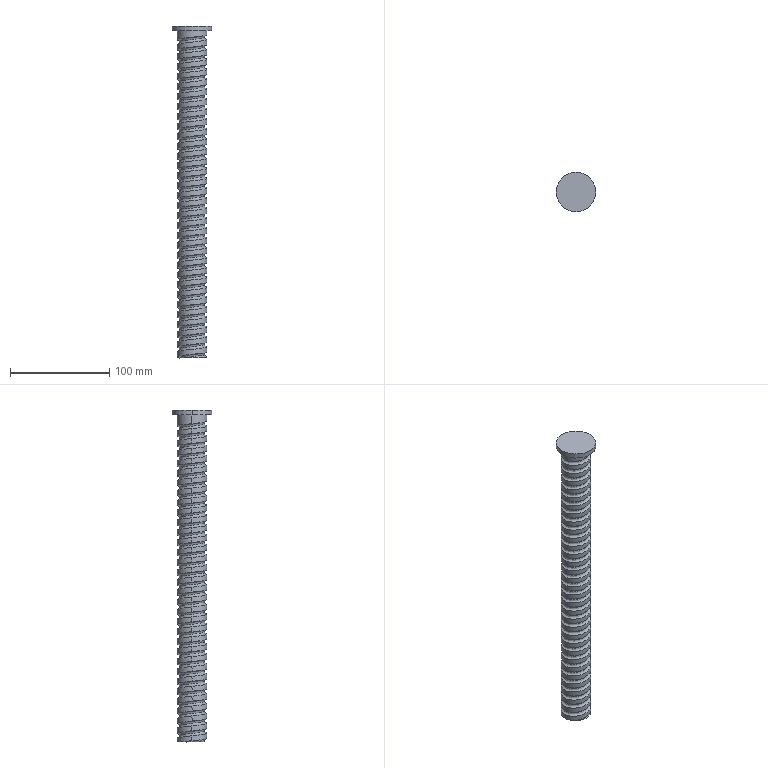Part | SolidWorks | features Extrusion 1, Helix 1, ICE 1, SweepCut 1 | 1 solid | 75 faces | box 40 x 40 x 335 mm | volume 211445 mm3 | cylinder 69 | plane 4 | spline 2 | commonest cylinder face diameters 30 x67 40 x2